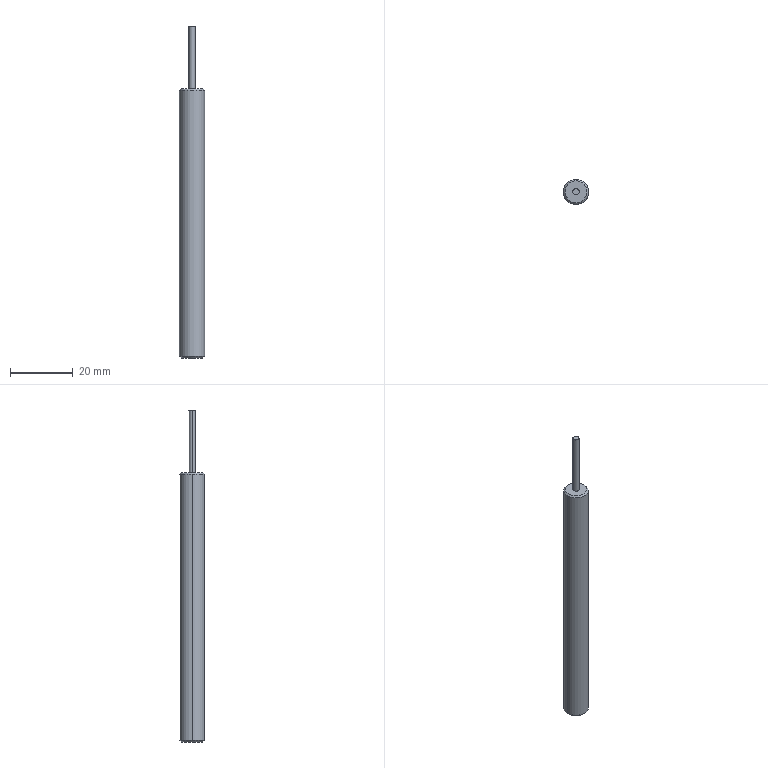Part | STEP file | 2064 Heating tube | 1 solid | 11 faces | box 8 x 8 x 106 mm | volume 4380 mm3 | cone 4 | cylinder 4 | plane 3 | commonest cylinder face diameters 2 x2 8 x2
STEP:
#1=CARTESIAN_POINT('',(0.,0.,0.));
#2=DIRECTION('',(0.,0.,1.));
#3=DIRECTION('',(1.,0.,0.));
#4=AXIS2_PLACEMENT_3D('',#1,#2,#3);
#5=CARTESIAN_POINT('',(-3.5,0.,0.));
#6=VERTEX_POINT('',#5);
#7=CARTESIAN_POINT('',(3.5,0.,0.));
#8=VERTEX_POINT('',#7);
#9=CARTESIAN_POINT('',(0.,0.,0.));
#10=DIRECTION('',(0.,0.,-1.));
#11=DIRECTION('',(1.,0.,0.));
#12=AXIS2_PLACEMENT_3D('',#9,#10,#11);
#13=CIRCLE('',#12,3.5);
#14=CARTESIAN_POINT('',(0.,0.,0.5));
#15=DIRECTION('',(0.,0.,1.));
#16=DIRECTION('',(1.,0.,0.));
#17=AXIS2_PLACEMENT_3D('',#14,#15,#16);
#18=CONICAL_SURFACE('',#17,4.,0.7854);
#19=CARTESIAN_POINT('',(6.283,-0.5));
#20=DIRECTION('',(-1.,0.));
#21=VECTOR('',#20,1.);
#22=LINE('',#19,#21);
#23=(GEOMETRIC_REPRESENTATION_CONTEXT(2)PARAMETRIC_REPRESENTATION_CONTEXT()REPRESENTATION_CONTEXT('',''));
#24=DEFINITIONAL_REPRESENTATION('',(#22),#23);
#25=PCURVE('',#18,#24);
#26=CARTESIAN_POINT('',(0.,0.,0.));
#27=DIRECTION('',(0.,0.,1.));
#28=DIRECTION('',(1.,0.,0.));
#29=AXIS2_PLACEMENT_3D('',#26,#27,#28);
#30=PLANE('',#29);
#31=CARTESIAN_POINT('',(3.5,0.));
#32=CARTESIAN_POINT('',(3.5,-6.062));
#33=CARTESIAN_POINT('',(-1.75,-3.031));
#34=CARTESIAN_POINT('',(-7.,0.));
#35=CARTESIAN_POINT('',(-1.75,3.031));
#36=CARTESIAN_POINT('',(3.5,6.062));
#37=CARTESIAN_POINT('',(3.5,0.));
#38=(BOUNDED_CURVE()B_SPLINE_CURVE(2,(#31,#32,#33,#34,#35,#36,#37),.UNSPECIFIED.,.T.,.F.)B_SPLINE_CURVE_WITH_KNOTS((1,2,2,2,2,1),(-2.094,0.,2.094,4.189,6.283,8.378),.UNSPECIFIED.)CURVE()GEOMETRIC_REPRESENTATION_ITEM()RATIONAL_B_SPLINE_CURVE((1.,0.5,1.,0.5,1.,0.5,1.))REPRESENTATION_ITEM(''));
#39=(GEOMETRIC_REPRESENTATION_CONTEXT(2)PARAMETRIC_REPRESENTATION_CONTEXT()REPRESENTATION_CONTEXT('',''));
#40=DEFINITIONAL_REPRESENTATION('',(#38),#39);
#41=PCURVE('',#30,#40);
#42=SURFACE_CURVE('',#13,(#25,#41),.PCURVE_S1.);
#43=EDGE_CURVE('',#6,#8,#42,.T.);
#44=ORIENTED_EDGE('',*,*,#43,.F.);
#45=CARTESIAN_POINT('',(-4.,0.,0.5));
#46=VERTEX_POINT('',#45);
#47=CARTESIAN_POINT('',(-4.,0.,0.5));
#48=DIRECTION('',(-0.7071,0.,0.7071));
#49=VECTOR('',#48,1.);
#50=LINE('',#47,#49);
#51=CARTESIAN_POINT('',(3.142,0.));
#52=DIRECTION('',(0.,1.));
#53=VECTOR('',#52,1.);
#54=LINE('',#51,#53);
#55=(GEOMETRIC_REPRESENTATION_CONTEXT(2)PARAMETRIC_REPRESENTATION_CONTEXT()REPRESENTATION_CONTEXT('',''));
#56=DEFINITIONAL_REPRESENTATION('',(#54),#55);
#57=PCURVE('',#18,#56);
#58=CARTESIAN_POINT('',(0.,0.,0.5));
#59=DIRECTION('',(0.,0.,1.));
#60=DIRECTION('',(1.,0.,0.));
#61=AXIS2_PLACEMENT_3D('',#58,#59,#60);
#62=CONICAL_SURFACE('',#61,4.,0.7854);
#63=CARTESIAN_POINT('',(3.142,0.));
#64=DIRECTION('',(0.,1.));
#65=VECTOR('',#64,1.);
#66=LINE('',#63,#65);
#67=(GEOMETRIC_REPRESENTATION_CONTEXT(2)PARAMETRIC_REPRESENTATION_CONTEXT()REPRESENTATION_CONTEXT('',''));
#68=DEFINITIONAL_REPRESENTATION('',(#66),#67);
#69=PCURVE('',#62,#68);
#70=SURFACE_CURVE('',#50,(#57,#69),.PCURVE_S1.);
#71=EDGE_CURVE('',#6,#46,#70,.T.);
#72=ORIENTED_EDGE('',*,*,#71,.T.);
#73=CARTESIAN_POINT('',(4.,0.,0.5));
#74=VERTEX_POINT('',#73);
#75=CARTESIAN_POINT('',(0.,0.,0.5));
#76=DIRECTION('',(0.,0.,1.));
#77=DIRECTION('',(1.,0.,0.));
#78=AXIS2_PLACEMENT_3D('',#75,#76,#77);
#79=CIRCLE('',#78,4.);
#80=CARTESIAN_POINT('',(0.,0.));
#81=DIRECTION('',(1.,0.));
#82=VECTOR('',#81,1.);
#83=LINE('',#80,#82);
#84=(GEOMETRIC_REPRESENTATION_CONTEXT(2)PARAMETRIC_REPRESENTATION_CONTEXT()REPRESENTATION_CONTEXT('',''));
#85=DEFINITIONAL_REPRESENTATION('',(#83),#84);
#86=PCURVE('',#18,#85);
#87=CARTESIAN_POINT('',(0.,0.,86.));
#88=DIRECTION('',(0.,0.,-1.));
#89=DIRECTION('',(-1.,0.,0.));
#90=AXIS2_PLACEMENT_3D('',#87,#88,#89);
#91=CYLINDRICAL_SURFACE('',#90,4.);
#92=CARTESIAN_POINT('',(3.142,85.5));
#93=DIRECTION('',(-1.,0.));
#94=VECTOR('',#93,1.);
#95=LINE('',#92,#94);
#96=(GEOMETRIC_REPRESENTATION_CONTEXT(2)PARAMETRIC_REPRESENTATION_CONTEXT()REPRESENTATION_CONTEXT('',''));
#97=DEFINITIONAL_REPRESENTATION('',(#95),#96);
#98=PCURVE('',#91,#97);
#99=SURFACE_CURVE('',#79,(#86,#98),.PCURVE_S1.);
#100=EDGE_CURVE('',#74,#46,#99,.T.);
#101=ORIENTED_EDGE('',*,*,#100,.F.);
#102=CARTESIAN_POINT('',(4.,0.,0.5));
#103=DIRECTION('',(0.7071,0.,0.7071));
#104=VECTOR('',#103,1.);
#105=LINE('',#102,#104);
#106=CARTESIAN_POINT('',(0.,0.));
#107=DIRECTION('',(0.,1.));
#108=VECTOR('',#107,1.);
#109=LINE('',#106,#108);
#110=(GEOMETRIC_REPRESENTATION_CONTEXT(2)PARAMETRIC_REPRESENTATION_CONTEXT()REPRESENTATION_CONTEXT('',''));
#111=DEFINITIONAL_REPRESENTATION('',(#109),#110);
#112=PCURVE('',#18,#111);
#113=CARTESIAN_POINT('',(6.283,0.));
#114=DIRECTION('',(0.,1.));
#115=VECTOR('',#114,1.);
#116=LINE('',#113,#115);
#117=(GEOMETRIC_REPRESENTATION_CONTEXT(2)PARAMETRIC_REPRESENTATION_CONTEXT()REPRESENTATION_CONTEXT('',''));
#118=DEFINITIONAL_REPRESENTATION('',(#116),#117);
#119=PCURVE('',#62,#118);
#120=SURFACE_CURVE('',#105,(#112,#119),.PCURVE_S1.);
#121=EDGE_CURVE('',#8,#74,#120,.T.);
#122=ORIENTED_EDGE('',*,*,#121,.F.);
#123=EDGE_LOOP('',(#44,#72,#101,#122));
#124=FACE_BOUND('',#123,.T.);
#125=ADVANCED_FACE('',(#124),#18,.T.);
#126=CARTESIAN_POINT('',(3.5,0.,86.));
#127=VERTEX_POINT('',#126);
#128=CARTESIAN_POINT('',(-3.5,0.,86.));
#129=VERTEX_POINT('',#128);
#130=CARTESIAN_POINT('',(0.,0.,86.));
#131=DIRECTION('',(0.,0.,1.));
#132=DIRECTION('',(1.,0.,0.));
#133=AXIS2_PLACEMENT_3D('',#130,#131,#132);
#134=CIRCLE('',#133,3.5);
#135=CARTESIAN_POINT('',(0.,0.,86.));
#136=DIRECTION('',(0.,0.,-1.));
#137=DIRECTION('',(-1.,0.,0.));
#138=AXIS2_PLACEMENT_3D('',#135,#136,#137);
#139=CONICAL_SURFACE('',#138,3.5,0.7854);
#140=CARTESIAN_POINT('',(3.142,0.));
#141=DIRECTION('',(-1.,0.));
#142=VECTOR('',#141,1.);
#143=LINE('',#140,#142);
#144=(GEOMETRIC_REPRESENTATION_CONTEXT(2)PARAMETRIC_REPRESENTATION_CONTEXT()REPRESENTATION_CONTEXT('',''));
#145=DEFINITIONAL_REPRESENTATION('',(#143),#144);
#146=PCURVE('',#139,#145);
#147=CARTESIAN_POINT('',(0.,0.,86.));
#148=DIRECTION('',(0.,0.,1.));
#149=DIRECTION('',(1.,0.,0.));
#150=AXIS2_PLACEMENT_3D('',#147,#148,#149);
#151=PLANE('',#150);
#152=CARTESIAN_POINT('',(0.,0.));
#153=DIRECTION('',(1.,0.));
#154=AXIS2_PLACEMENT_2D('',#152,#153);
#155=CIRCLE('',#154,3.5);
#156=(GEOMETRIC_REPRESENTATION_CONTEXT(2)PARAMETRIC_REPRESENTATION_CONTEXT()REPRESENTATION_CONTEXT('',''));
#157=DEFINITIONAL_REPRESENTATION('',(#155),#156);
#158=PCURVE('',#151,#157);
#159=SURFACE_CURVE('',#134,(#146,#158),.PCURVE_S1.);
#160=EDGE_CURVE('',#127,#129,#159,.T.);
#161=ORIENTED_EDGE('',*,*,#160,.F.);
#162=CARTESIAN_POINT('',(4.,0.,85.5));
#163=VERTEX_POINT('',#162);
#164=CARTESIAN_POINT('',(3.5,0.,86.));
#165=DIRECTION('',(0.7071,0.,-0.7071));
#166=VECTOR('',#165,1.);
#167=LINE('',#164,#166);
#168=CARTESIAN_POINT('',(3.142,0.));
#169=DIRECTION('',(0.,1.));
#170=VECTOR('',#169,1.);
#171=LINE('',#168,#170);
#172=(GEOMETRIC_REPRESENTATION_CONTEXT(2)PARAMETRIC_REPRESENTATION_CONTEXT()REPRESENTATION_CONTEXT('',''));
#173=DEFINITIONAL_REPRESENTATION('',(#171),#172);
#174=PCURVE('',#139,#173);
#175=CARTESIAN_POINT('',(0.,0.,86.));
#176=DIRECTION('',(0.,0.,-1.));
#177=DIRECTION('',(-1.,0.,0.));
#178=AXIS2_PLACEMENT_3D('',#175,#176,#177);
#179=CONICAL_SURFACE('',#178,3.5,0.7854);
#180=CARTESIAN_POINT('',(3.142,0.));
#181=DIRECTION('',(0.,1.));
#182=VECTOR('',#181,1.);
#183=LINE('',#180,#182);
#184=(GEOMETRIC_REPRESENTATION_CONTEXT(2)PARAMETRIC_REPRESENTATION_CONTEXT()REPRESENTATION_CONTEXT('',''));
#185=DEFINITIONAL_REPRESENTATION('',(#183),#184);
#186=PCURVE('',#179,#185);
#187=SURFACE_CURVE('',#167,(#174,#186),.PCURVE_S1.);
#188=EDGE_CURVE('',#127,#163,#187,.T.);
#189=ORIENTED_EDGE('',*,*,#188,.T.);
#190=CARTESIAN_POINT('',(-4.,0.,85.5));
#191=VERTEX_POINT('',#190);
#192=CARTESIAN_POINT('',(0.,0.,85.5));
#193=DIRECTION('',(0.,0.,-1.));
#194=DIRECTION('',(1.,0.,0.));
#195=AXIS2_PLACEMENT_3D('',#192,#193,#194);
#196=CIRCLE('',#195,4.);
#197=CARTESIAN_POINT('',(-3.142,0.5));
#198=DIRECTION('',(1.,0.));
#199=VECTOR('',#198,1.);
#200=LINE('',#197,#199);
#201=(GEOMETRIC_REPRESENTATION_CONTEXT(2)PARAMETRIC_REPRESENTATION_CONTEXT()REPRESENTATION_CONTEXT('',''));
#202=DEFINITIONAL_REPRESENTATION('',(#200),#201);
#203=PCURVE('',#139,#202);
#204=CARTESIAN_POINT('',(-3.142,0.5));
#205=DIRECTION('',(1.,0.));
#206=VECTOR('',#205,1.);
#207=LINE('',#204,#206);
#208=(GEOMETRIC_REPRESENTATION_CONTEXT(2)PARAMETRIC_REPRESENTATION_CONTEXT()REPRESENTATION_CONTEXT('',''));
#209=DEFINITIONAL_REPRESENTATION('',(#207),#208);
#210=PCURVE('',#91,#209);
#211=SURFACE_CURVE('',#196,(#203,#210),.PCURVE_S1.);
#212=EDGE_CURVE('',#191,#163,#211,.T.);
#213=ORIENTED_EDGE('',*,*,#212,.F.);
#214=CARTESIAN_POINT('',(-3.5,0.,86.));
#215=DIRECTION('',(-0.7071,0.,-0.7071));
#216=VECTOR('',#215,1.);
#217=LINE('',#214,#216);
#218=CARTESIAN_POINT('',(0.,0.));
#219=DIRECTION('',(0.,1.));
#220=VECTOR('',#219,1.);
#221=LINE('',#218,#220);
#222=(GEOMETRIC_REPRESENTATION_CONTEXT(2)PARAMETRIC_REPRESENTATION_CONTEXT()REPRESENTATION_CONTEXT('',''));
#223=DEFINITIONAL_REPRESENTATION('',(#221),#222);
#224=PCURVE('',#139,#223);
#225=CARTESIAN_POINT('',(6.283,0.));
#226=DIRECTION('',(0.,1.));
#227=VECTOR('',#226,1.);
#228=LINE('',#225,#227);
#229=(GEOMETRIC_REPRESENTATION_CONTEXT(2)PARAMETRIC_REPRESENTATION_CONTEXT()REPRESENTATION_CONTEXT('',''));
#230=DEFINITIONAL_REPRESENTATION('',(#228),#229);
#231=PCURVE('',#179,#230);
#232=SURFACE_CURVE('',#217,(#224,#231),.PCURVE_S1.);
#233=EDGE_CURVE('',#129,#191,#232,.T.);
#234=ORIENTED_EDGE('',*,*,#233,.F.);
#235=EDGE_LOOP('',(#161,#189,#213,#234));
#236=FACE_BOUND('',#235,.T.);
#237=ADVANCED_FACE('',(#236),#139,.T.);
#238=CARTESIAN_POINT('',(1.,0.,106.));
#239=VERTEX_POINT('',#238);
#240=CARTESIAN_POINT('',(-1.,0.,106.));
#241=VERTEX_POINT('',#240);
#242=CARTESIAN_POINT('',(0.,0.,106.));
#243=DIRECTION('',(0.,0.,1.));
#244=DIRECTION('',(1.,0.,0.));
#245=AXIS2_PLACEMENT_3D('',#242,#243,#244);
#246=CIRCLE('',#245,1.);
#247=CARTESIAN_POINT('',(0.,0.,106.));
#248=DIRECTION('',(0.,0.,-1.));
#249=DIRECTION('',(-1.,0.,0.));
#250=AXIS2_PLACEMENT_3D('',#247,#248,#249);
#251=CYLINDRICAL_SURFACE('',#250,1.);
#252=CARTESIAN_POINT('',(3.142,0.));
#253=DIRECTION('',(-1.,0.));
#254=VECTOR('',#253,1.);
#255=LINE('',#252,#254);
#256=(GEOMETRIC_REPRESENTATION_CONTEXT(2)PARAMETRIC_REPRESENTATION_CONTEXT()REPRESENTATION_CONTEXT('',''));
#257=DEFINITIONAL_REPRESENTATION('',(#255),#256);
#258=PCURVE('',#251,#257);
#259=CARTESIAN_POINT('',(0.,0.,106.));
#260=DIRECTION('',(0.,0.,1.));
#261=DIRECTION('',(1.,0.,0.));
#262=AXIS2_PLACEMENT_3D('',#259,#260,#261);
#263=PLANE('',#262);
#264=CARTESIAN_POINT('',(0.,0.));
#265=DIRECTION('',(1.,0.));
#266=AXIS2_PLACEMENT_2D('',#264,#265);
#267=CIRCLE('',#266,1.);
#268=(GEOMETRIC_REPRESENTATION_CONTEXT(2)PARAMETRIC_REPRESENTATION_CONTEXT()REPRESENTATION_CONTEXT('',''));
#269=DEFINITIONAL_REPRESENTATION('',(#267),#268);
#270=PCURVE('',#263,#269);
#271=SURFACE_CURVE('',#246,(#258,#270),.PCURVE_S1.);
#272=EDGE_CURVE('',#239,#241,#271,.T.);
#273=ORIENTED_EDGE('',*,*,#272,.F.);
#274=CARTESIAN_POINT('',(1.,0.,86.));
#275=VERTEX_POINT('',#274);
#276=CARTESIAN_POINT('',(1.,0.,106.));
#277=DIRECTION('',(0.,0.,-1.));
#278=VECTOR('',#277,1.);
#279=LINE('',#276,#278);
#280=CARTESIAN_POINT('',(3.142,0.));
#281=DIRECTION('',(0.,1.));
#282=VECTOR('',#281,1.);
#283=LINE('',#280,#282);
#284=(GEOMETRIC_REPRESENTATION_CONTEXT(2)PARAMETRIC_REPRESENTATION_CONTEXT()REPRESENTATION_CONTEXT('',''));
#285=DEFINITIONAL_REPRESENTATION('',(#283),#284);
#286=PCURVE('',#251,#285);
#287=CARTESIAN_POINT('',(0.,0.,106.));
#288=DIRECTION('',(0.,0.,-1.));
#289=DIRECTION('',(-1.,0.,0.));
#290=AXIS2_PLACEMENT_3D('',#287,#288,#289);
#291=CYLINDRICAL_SURFACE('',#290,1.);
#292=CARTESIAN_POINT('',(3.142,0.));
#293=DIRECTION('',(0.,1.));
#294=VECTOR('',#293,1.);
#295=LINE('',#292,#294);
#296=(GEOMETRIC_REPRESENTATION_CONTEXT(2)PARAMETRIC_REPRESENTATION_CONTEXT()REPRESENTATION_CONTEXT('',''));
#297=DEFINITIONAL_REPRESENTATION('',(#295),#296);
#298=PCURVE('',#291,#297);
#299=SURFACE_CURVE('',#279,(#286,#298),.PCURVE_S1.);
#300=EDGE_CURVE('',#239,#275,#299,.T.);
#301=ORIENTED_EDGE('',*,*,#300,.T.);
#302=CARTESIAN_POINT('',(-1.,0.,86.));
#303=VERTEX_POINT('',#302);
#304=CARTESIAN_POINT('',(0.,0.,86.));
#305=DIRECTION('',(0.,0.,1.));
#306=DIRECTION('',(1.,0.,0.));
#307=AXIS2_PLACEMENT_3D('',#304,#305,#306);
#308=CIRCLE('',#307,1.);
#309=CARTESIAN_POINT('',(3.142,20.));
#310=DIRECTION('',(-1.,0.));
#311=VECTOR('',#310,1.);
#312=LINE('',#309,#311);
#313=(GEOMETRIC_REPRESENTATION_CONTEXT(2)PARAMETRIC_REPRESENTATION_CONTEXT()REPRESENTATION_CONTEXT('',''));
#314=DEFINITIONAL_REPRESENTATION('',(#312),#313);
#315=PCURVE('',#251,#314);
#316=CARTESIAN_POINT('',(0.,0.));
#317=DIRECTION('',(1.,0.));
#318=AXIS2_PLACEMENT_2D('',#316,#317);
#319=CIRCLE('',#318,1.);
#320=(GEOMETRIC_REPRESENTATION_CONTEXT(2)PARAMETRIC_REPRESENTATION_CONTEXT()REPRESENTATION_CONTEXT('',''));
#321=DEFINITIONAL_REPRESENTATION('',(#319),#320);
#322=PCURVE('',#151,#321);
#323=SURFACE_CURVE('',#308,(#315,#322),.PCURVE_S1.);
#324=EDGE_CURVE('',#275,#303,#323,.T.);
#325=ORIENTED_EDGE('',*,*,#324,.T.);
#326=CARTESIAN_POINT('',(-1.,0.,106.));
#327=DIRECTION('',(0.,0.,-1.));
#328=VECTOR('',#327,1.);
#329=LINE('',#326,#328);
#330=CARTESIAN_POINT('',(0.,0.));
#331=DIRECTION('',(0.,1.));
#332=VECTOR('',#331,1.);
#333=LINE('',#330,#332);
#334=(GEOMETRIC_REPRESENTATION_CONTEXT(2)PARAMETRIC_REPRESENTATION_CONTEXT()REPRESENTATION_CONTEXT('',''));
#335=DEFINITIONAL_REPRESENTATION('',(#333),#334);
#336=PCURVE('',#251,#335);
#337=CARTESIAN_POINT('',(6.283,0.));
#338=DIRECTION('',(0.,1.));
#339=VECTOR('',#338,1.);
#340=LINE('',#337,#339);
#341=(GEOMETRIC_REPRESENTATION_CONTEXT(2)PARAMETRIC_REPRESENTATION_CONTEXT()REPRESENTATION_CONTEXT('',''));
#342=DEFINITIONAL_REPRESENTATION('',(#340),#341);
#343=PCURVE('',#291,#342);
#344=SURFACE_CURVE('',#329,(#336,#343),.PCURVE_S1.);
#345=EDGE_CURVE('',#241,#303,#344,.T.);
#346=ORIENTED_EDGE('',*,*,#345,.F.);
#347=EDGE_LOOP('',(#273,#301,#325,#346));
#348=FACE_BOUND('',#347,.T.);
#349=ADVANCED_FACE('',(#348),#251,.T.);
#350=ORIENTED_EDGE('',*,*,#212,.T.);
#351=CARTESIAN_POINT('',(4.,0.,86.));
#352=DIRECTION('',(0.,0.,-1.));
#353=VECTOR('',#352,1.);
#354=LINE('',#351,#353);
#355=CARTESIAN_POINT('',(3.142,0.));
#356=DIRECTION('',(0.,1.));
#357=VECTOR('',#356,1.);
#358=LINE('',#355,#357);
#359=(GEOMETRIC_REPRESENTATION_CONTEXT(2)PARAMETRIC_REPRESENTATION_CONTEXT()REPRESENTATION_CONTEXT('',''));
#360=DEFINITIONAL_REPRESENTATION('',(#358),#359);
#361=PCURVE('',#91,#360);
#362=CARTESIAN_POINT('',(0.,0.,86.));
#363=DIRECTION('',(0.,0.,-1.));
#364=DIRECTION('',(-1.,0.,0.));
#365=AXIS2_PLACEMENT_3D('',#362,#363,#364);
#366=CYLINDRICAL_SURFACE('',#365,4.);
#367=CARTESIAN_POINT('',(3.142,0.));
#368=DIRECTION('',(0.,1.));
#369=VECTOR('',#368,1.);
#370=LINE('',#367,#369);
#371=(GEOMETRIC_REPRESENTATION_CONTEXT(2)PARAMETRIC_REPRESENTATION_CONTEXT()REPRESENTATION_CONTEXT('',''));
#372=DEFINITIONAL_REPRESENTATION('',(#370),#371);
#373=PCURVE('',#366,#372);
#374=SURFACE_CURVE('',#354,(#361,#373),.PCURVE_S1.);
#375=EDGE_CURVE('',#163,#74,#374,.T.);
#376=ORIENTED_EDGE('',*,*,#375,.T.);
#377=ORIENTED_EDGE('',*,*,#100,.T.);
#378=CARTESIAN_POINT('',(-4.,0.,86.));
#379=DIRECTION('',(0.,0.,-1.));
#380=VECTOR('',#379,1.);
#381=LINE('',#378,#380);
#382=CARTESIAN_POINT('',(0.,0.));
#383=DIRECTION('',(0.,1.));
#384=VECTOR('',#383,1.);
#385=LINE('',#382,#384);
#386=(GEOMETRIC_REPRESENTATION_CONTEXT(2)PARAMETRIC_REPRESENTATION_CONTEXT()REPRESENTATION_CONTEXT('',''));
#387=DEFINITIONAL_REPRESENTATION('',(#385),#386);
#388=PCURVE('',#91,#387);
#389=CARTESIAN_POINT('',(6.283,0.));
#390=DIRECTION('',(0.,1.));
#391=VECTOR('',#390,1.);
#392=LINE('',#389,#391);
#393=(GEOMETRIC_REPRESENTATION_CONTEXT(2)PARAMETRIC_REPRESENTATION_CONTEXT()REPRESENTATION_CONTEXT('',''));
#394=DEFINITIONAL_REPRESENTATION('',(#392),#393);
#395=PCURVE('',#366,#394);
#396=SURFACE_CURVE('',#381,(#388,#395),.PCURVE_S1.);
#397=EDGE_CURVE('',#191,#46,#396,.T.);
#398=ORIENTED_EDGE('',*,*,#397,.F.);
#399=EDGE_LOOP('',(#350,#376,#377,#398));
#400=FACE_BOUND('',#399,.T.);
#401=ADVANCED_FACE('',(#400),#91,.T.);
#402=CARTESIAN_POINT('',(0.,0.,86.));
#403=DIRECTION('',(0.,0.,1.));
#404=DIRECTION('',(1.,0.,0.));
#405=AXIS2_PLACEMENT_3D('',#402,#403,#404);
#406=CIRCLE('',#405,3.5);
#407=CARTESIAN_POINT('',(0.,0.));
#408=DIRECTION('',(1.,0.));
#409=AXIS2_PLACEMENT_2D('',#407,#408);
#410=CIRCLE('',#409,3.5);
#411=(GEOMETRIC_REPRESENTATION_CONTEXT(2)PARAMETRIC_REPRESENTATION_CONTEXT()REPRESENTATION_CONTEXT('',''));
#412=DEFINITIONAL_REPRESENTATION('',(#410),#411);
#413=PCURVE('',#151,#412);
#414=CARTESIAN_POINT('',(9.425,0.));
#415=DIRECTION('',(-1.,0.));
#416=VECTOR('',#415,1.);
#417=LINE('',#414,#416);
#418=(GEOMETRIC_REPRESENTATION_CONTEXT(2)PARAMETRIC_REPRESENTATION_CONTEXT()REPRESENTATION_CONTEXT('',''));
#419=DEFINITIONAL_REPRESENTATION('',(#417),#418);
#420=PCURVE('',#179,#419);
#421=SURFACE_CURVE('',#406,(#413,#420),.PCURVE_S1.);
#422=EDGE_CURVE('',#129,#127,#421,.T.);
#423=ORIENTED_EDGE('',*,*,#422,.T.);
#424=ORIENTED_EDGE('',*,*,#160,.T.);
#425=EDGE_LOOP('',(#423,#424));
#426=FACE_BOUND('',#425,.T.);
#427=CARTESIAN_POINT('',(0.,0.,86.));
#428=DIRECTION('',(0.,0.,1.));
#429=DIRECTION('',(1.,0.,0.));
#430=AXIS2_PLACEMENT_3D('',#427,#428,#429);
#431=CIRCLE('',#430,1.);
#432=CARTESIAN_POINT('',(0.,0.));
#433=DIRECTION('',(1.,0.));
#434=AXIS2_PLACEMENT_2D('',#432,#433);
#435=CIRCLE('',#434,1.);
#436=(GEOMETRIC_REPRESENTATION_CONTEXT(2)PARAMETRIC_REPRESENTATION_CONTEXT()REPRESENTATION_CONTEXT('',''));
#437=DEFINITIONAL_REPRESENTATION('',(#435),#436);
#438=PCURVE('',#151,#437);
#439=CARTESIAN_POINT('',(9.425,20.));
#440=DIRECTION('',(-1.,0.));
#441=VECTOR('',#440,1.);
#442=LINE('',#439,#441);
#443=(GEOMETRIC_REPRESENTATION_CONTEXT(2)PARAMETRIC_REPRESENTATION_CONTEXT()REPRESENTATION_CONTEXT('',''));
#444=DEFINITIONAL_REPRESENTATION('',(#442),#443);
#445=PCURVE('',#291,#444);
#446=SURFACE_CURVE('',#431,(#438,#445),.PCURVE_S1.);
#447=EDGE_CURVE('',#303,#275,#446,.T.);
#448=ORIENTED_EDGE('',*,*,#447,.F.);
#449=ORIENTED_EDGE('',*,*,#324,.F.);
#450=EDGE_LOOP('',(#448,#449));
#451=FACE_BOUND('',#450,.T.);
#452=ADVANCED_FACE('',(#426,#451),#151,.T.);
#453=ORIENTED_EDGE('',*,*,#375,.F.);
#454=CARTESIAN_POINT('',(0.,0.,85.5));
#455=DIRECTION('',(0.,0.,-1.));
#456=DIRECTION('',(1.,0.,0.));
#457=AXIS2_PLACEMENT_3D('',#454,#455,#456);
#458=CIRCLE('',#457,4.);
#459=CARTESIAN_POINT('',(3.142,0.5));
#460=DIRECTION('',(1.,0.));
#461=VECTOR('',#460,1.);
#462=LINE('',#459,#461);
#463=(GEOMETRIC_REPRESENTATION_CONTEXT(2)PARAMETRIC_REPRESENTATION_CONTEXT()REPRESENTATION_CONTEXT('',''));
#464=DEFINITIONAL_REPRESENTATION('',(#462),#463);
#465=PCURVE('',#366,#464);
#466=CARTESIAN_POINT('',(3.142,0.5));
#467=DIRECTION('',(1.,0.));
#468=VECTOR('',#467,1.);
#469=LINE('',#466,#468);
#470=(GEOMETRIC_REPRESENTATION_CONTEXT(2)PARAMETRIC_REPRESENTATION_CONTEXT()REPRESENTATION_CONTEXT('',''));
#471=DEFINITIONAL_REPRESENTATION('',(#469),#470);
#472=PCURVE('',#179,#471);
#473=SURFACE_CURVE('',#458,(#465,#472),.PCURVE_S1.);
#474=EDGE_CURVE('',#163,#191,#473,.T.);
#475=ORIENTED_EDGE('',*,*,#474,.T.);
#476=ORIENTED_EDGE('',*,*,#397,.T.);
#477=CARTESIAN_POINT('',(0.,0.,0.5));
#478=DIRECTION('',(0.,0.,1.));
#479=DIRECTION('',(1.,0.,0.));
#480=AXIS2_PLACEMENT_3D('',#477,#478,#479);
#481=CIRCLE('',#480,4.);
#482=CARTESIAN_POINT('',(9.425,85.5));
#483=DIRECTION('',(-1.,0.));
#484=VECTOR('',#483,1.);
#485=LINE('',#482,#484);
#486=(GEOMETRIC_REPRESENTATION_CONTEXT(2)PARAMETRIC_REPRESENTATION_CONTEXT()REPRESENTATION_CONTEXT('',''));
#487=DEFINITIONAL_REPRESENTATION('',(#485),#486);
#488=PCURVE('',#366,#487);
#489=CARTESIAN_POINT('',(0.,0.));
#490=DIRECTION('',(1.,0.));
#491=VECTOR('',#490,1.);
#492=LINE('',#489,#491);
#493=(GEOMETRIC_REPRESENTATION_CONTEXT(2)PARAMETRIC_REPRESENTATION_CONTEXT()REPRESENTATION_CONTEXT('',''));
#494=DEFINITIONAL_REPRESENTATION('',(#492),#493);
#495=PCURVE('',#62,#494);
#496=SURFACE_CURVE('',#481,(#488,#495),.PCURVE_S1.);
#497=EDGE_CURVE('',#46,#74,#496,.T.);
#498=ORIENTED_EDGE('',*,*,#497,.T.);
#499=EDGE_LOOP('',(#453,#475,#476,#498));
#500=FACE_BOUND('',#499,.T.);
#501=ADVANCED_FACE('',(#500),#366,.T.);
#502=CARTESIAN_POINT('',(0.,0.,0.));
#503=DIRECTION('',(0.,0.,-1.));
#504=DIRECTION('',(1.,0.,0.));
#505=AXIS2_PLACEMENT_3D('',#502,#503,#504);
#506=CIRCLE('',#505,3.5);
#507=CARTESIAN_POINT('',(3.5,0.));
#508=CARTESIAN_POINT('',(3.5,-6.062));
#509=CARTESIAN_POINT('',(-1.75,-3.031));
#510=CARTESIAN_POINT('',(-7.,0.));
#511=CARTESIAN_POINT('',(-1.75,3.031));
#512=CARTESIAN_POINT('',(3.5,6.062));
#513=CARTESIAN_POINT('',(3.5,0.));
#514=(BOUNDED_CURVE()B_SPLINE_CURVE(2,(#507,#508,#509,#510,#511,#512,#513),.UNSPECIFIED.,.T.,.F.)B_SPLINE_CURVE_WITH_KNOTS((1,2,2,2,2,1),(-2.094,0.,2.094,4.189,6.283,8.378),.UNSPECIFIED.)CURVE()GEOMETRIC_REPRESENTATION_ITEM()RATIONAL_B_SPLINE_CURVE((1.,0.5,1.,0.5,1.,0.5,1.))REPRESENTATION_ITEM(''));
#515=(GEOMETRIC_REPRESENTATION_CONTEXT(2)PARAMETRIC_REPRESENTATION_CONTEXT()REPRESENTATION_CONTEXT('',''));
#516=DEFINITIONAL_REPRESENTATION('',(#514),#515);
#517=PCURVE('',#30,#516);
#518=CARTESIAN_POINT('',(6.283,-0.5));
#519=DIRECTION('',(-1.,0.));
#520=VECTOR('',#519,1.);
#521=LINE('',#518,#520);
#522=(GEOMETRIC_REPRESENTATION_CONTEXT(2)PARAMETRIC_REPRESENTATION_CONTEXT()REPRESENTATION_CONTEXT('',''));
#523=DEFINITIONAL_REPRESENTATION('',(#521),#522);
#524=PCURVE('',#62,#523);
#525=SURFACE_CURVE('',#506,(#517,#524),.PCURVE_S1.);
#526=EDGE_CURVE('',#8,#6,#525,.T.);
#527=ORIENTED_EDGE('',*,*,#526,.T.);
#528=ORIENTED_EDGE('',*,*,#43,.T.);
#529=EDGE_LOOP('',(#527,#528));
#530=FACE_BOUND('',#529,.T.);
#531=ADVANCED_FACE('',(#530),#30,.F.);
#532=ORIENTED_EDGE('',*,*,#300,.F.);
#533=CARTESIAN_POINT('',(0.,0.,106.));
#534=DIRECTION('',(0.,0.,1.));
#535=DIRECTION('',(1.,0.,0.));
#536=AXIS2_PLACEMENT_3D('',#533,#534,#535);
#537=CIRCLE('',#536,1.);
#538=CARTESIAN_POINT('',(9.425,0.));
#539=DIRECTION('',(-1.,0.));
#540=VECTOR('',#539,1.);
#541=LINE('',#538,#540);
#542=(GEOMETRIC_REPRESENTATION_CONTEXT(2)PARAMETRIC_REPRESENTATION_CONTEXT()REPRESENTATION_CONTEXT('',''));
#543=DEFINITIONAL_REPRESENTATION('',(#541),#542);
#544=PCURVE('',#291,#543);
#545=CARTESIAN_POINT('',(0.,0.));
#546=DIRECTION('',(1.,0.));
#547=AXIS2_PLACEMENT_2D('',#545,#546);
#548=CIRCLE('',#547,1.);
#549=(GEOMETRIC_REPRESENTATION_CONTEXT(2)PARAMETRIC_REPRESENTATION_CONTEXT()REPRESENTATION_CONTEXT('',''));
#550=DEFINITIONAL_REPRESENTATION('',(#548),#549);
#551=PCURVE('',#263,#550);
#552=SURFACE_CURVE('',#537,(#544,#551),.PCURVE_S1.);
#553=EDGE_CURVE('',#241,#239,#552,.T.);
#554=ORIENTED_EDGE('',*,*,#553,.F.);
#555=ORIENTED_EDGE('',*,*,#345,.T.);
#556=ORIENTED_EDGE('',*,*,#447,.T.);
#557=EDGE_LOOP('',(#532,#554,#555,#556));
#558=FACE_BOUND('',#557,.T.);
#559=ADVANCED_FACE('',(#558),#291,.T.);
#560=ORIENTED_EDGE('',*,*,#553,.T.);
#561=ORIENTED_EDGE('',*,*,#272,.T.);
#562=EDGE_LOOP('',(#560,#561));
#563=FACE_BOUND('',#562,.T.);
#564=ADVANCED_FACE('',(#563),#263,.T.);
#565=ORIENTED_EDGE('',*,*,#188,.F.);
#566=ORIENTED_EDGE('',*,*,#422,.F.);
#567=ORIENTED_EDGE('',*,*,#233,.T.);
#568=ORIENTED_EDGE('',*,*,#474,.F.);
#569=EDGE_LOOP('',(#565,#566,#567,#568));
#570=FACE_BOUND('',#569,.T.);
#571=ADVANCED_FACE('',(#570),#179,.T.);
#572=ORIENTED_EDGE('',*,*,#71,.F.);
#573=ORIENTED_EDGE('',*,*,#526,.F.);
#574=ORIENTED_EDGE('',*,*,#121,.T.);
#575=ORIENTED_EDGE('',*,*,#497,.F.);
#576=EDGE_LOOP('',(#572,#573,#574,#575));
#577=FACE_BOUND('',#576,.T.);
#578=ADVANCED_FACE('',(#577),#62,.T.);
#579=CLOSED_SHELL('',(#125,#237,#349,#401,#452,#501,#531,#559,#564,#571,#578));
#580=MANIFOLD_SOLID_BREP('',#579);
#581=(LENGTH_UNIT()NAMED_UNIT(*)SI_UNIT(.MILLI.,.METRE.));
#582=UNCERTAINTY_MEASURE_WITH_UNIT(LENGTH_MEASURE(0.0000001),#581,'','');
#583=(NAMED_UNIT(*)PLANE_ANGLE_UNIT()SI_UNIT($,.RADIAN.));
#584=(NAMED_UNIT(*)SI_UNIT($,.STERADIAN.)SOLID_ANGLE_UNIT());
#585=(GEOMETRIC_REPRESENTATION_CONTEXT(3)GLOBAL_UNCERTAINTY_ASSIGNED_CONTEXT((#582))GLOBAL_UNIT_ASSIGNED_CONTEXT((#581,#583,#584))REPRESENTATION_CONTEXT('',''));
#586=ADVANCED_BREP_SHAPE_REPRESENTATION('',(#4,#580),#585);